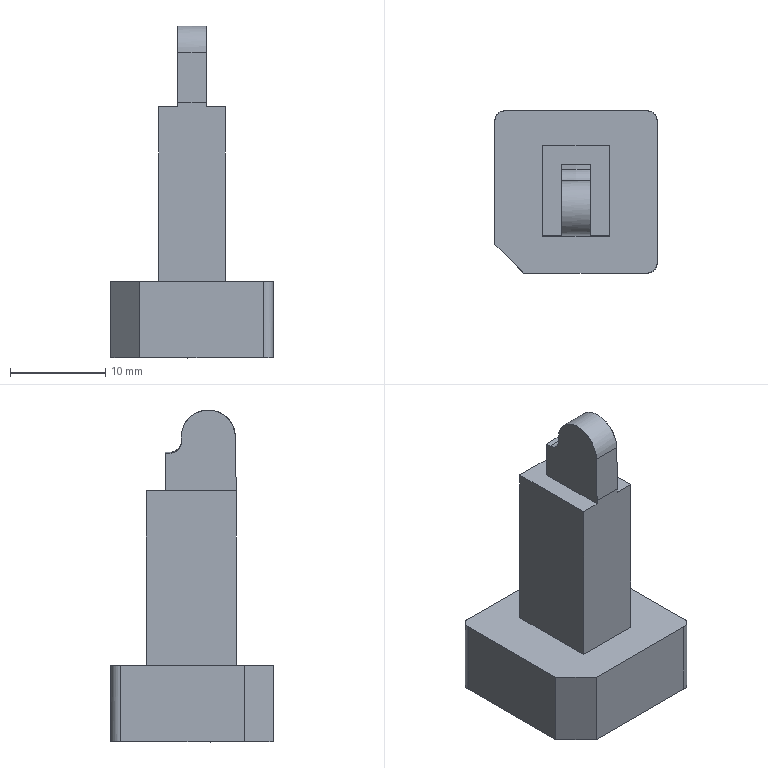NC program | PowerMill | posted with a generic post | part box 17 x 17 x 34.811 mm
Lines 6713 to 7479 of 35253:
N6810 M6
N6811 S18000 M03
N6812 G00 G90 X0.0 Y0.0
N6813 G43 Z10.798 H4
N6814
N6815 G05 P10000 R8
N6816 X1.6466 Y-5.3026
N6817 Z-2.4586
N6818 G01 Z-3.6586 F1200.0
N6819 X1.6444 Y-5.3048 Z-3.6763 F2000.0
N6820 X1.5692 Y-5.3292 Z-3.8957
N6821 X1.5752 Y-5.3231 Z-3.779
N6822 X1.587 Y-5.3114 Z-3.6547
N6823 X1.6045 Y-5.2939 Z-3.5284
N6824 X1.6264 Y-5.2719 Z-3.4092
N6825 X1.6518 Y-5.2466 Z-3.2995
N6826 X1.6598 Y-5.2386 Z-3.2691
N6827 X1.6694 Y-5.178 Z-3.0351
N6828 X1.6692 Y-5.1783 Z-3.0359
N6829 X1.635 Y-5.2125 Z-3.1368
N6830 X1.6045 Y-5.243 Z-3.245
N6831 X1.5779 Y-5.2696 Z-3.3607
N6832 X1.5553 Y-5.2921 Z-3.4838
N6833 X1.5372 Y-5.3102 Z-3.6141
N6834 X1.5238 Y-5.3236 Z-3.751
N6835 X1.5154 Y-5.332 Z-3.8931
N6836 X1.5123 Y-5.3352 Z-4.0382
N6837 X1.4611 Y-5.3355 Z-4.0525
N6838 X1.4638 Y-5.3327 Z-3.9138
N6839 X1.4717 Y-5.3248 Z-3.7684
N6840 X1.4849 Y-5.3117 Z-3.6241
N6841 X1.5029 Y-5.2936 Z-3.4852
N6842 X1.5253 Y-5.2712 Z-3.354
N6843 X1.5516 Y-5.2449 Z-3.2313
N6844 X1.5814 Y-5.2151 Z-3.1176
N6845 X1.6145 Y-5.1821 Z-3.0128
N6846 X1.6505 Y-5.1461 Z-2.9166
N6847 X1.6681 Y-5.1285 Z-2.8749
N6848 X1.6657 Y-5.0799 Z-2.7385
N6849 X1.6407 Y-5.1049 Z-2.7911
N6850 X1.6027 Y-5.1429 Z-2.8824
N6851 X1.5668 Y-5.1789 Z-2.9837
N6852 X1.5332 Y-5.2124 Z-3.0957
N6853 X1.5025 Y-5.2431 Z-3.2179
N6854 X1.4754 Y-5.2703 Z-3.3482
N6855 X1.4582 Y-5.2874 Z-3.447
N6856 X1.4406 Y-5.305 Z-3.5684
N6857 X1.4271 Y-5.3185 Z-3.6908
N6858 X1.4177 Y-5.328 Z-3.819
N6859 X1.4124 Y-5.3332 Z-3.9429
N6860 X1.4098 Y-5.3358 Z-4.0669
N6861 X1.3586 Y-5.3361 Z-4.0813
N6862 X1.3611 Y-5.3336 Z-3.9744
N6863 X1.3646 Y-5.3302 Z-3.8674
N6864 X1.3702 Y-5.3245 Z-3.7607
N6865 X1.3792 Y-5.3155 Z-3.6546
N6866 X1.392 Y-5.3028 Z-3.5494
N6867 X1.408 Y-5.2867 Z-3.445
N6868 X1.4262 Y-5.2685 Z-3.3433
N6869 X1.4553 Y-5.2394 Z-3.2034
N6870 X1.4875 Y-5.2073 Z-3.0738
N6871 X1.5223 Y-5.1724 Z-2.9551
N6872 X1.5596 Y-5.1351 Z-2.8467
N6873 X1.5994 Y-5.0953 Z-2.7478
N6874 X1.6416 Y-5.0531 Z-2.6579
N6875 X1.6679 Y-5.0269 Z-2.6085
N6876 X1.668 Y-4.9758 Z-2.495
N6877 X1.6354 Y-5.0084 Z-2.5489
N6878 X1.601 Y-5.0428 Z-2.6155
N6879 X1.5644 Y-5.0794 Z-2.6968
N6880 X1.5251 Y-5.1187 Z-2.7965
N6881 X1.4836 Y-5.1602 Z-2.9169
N6882 X1.4525 Y-5.1913 Z-3.0187
N6883 X1.4292 Y-5.2146 Z-3.1034
N6884 X1.4108 Y-5.233 Z-3.1767
N6885 X1.3834 Y-5.2604 Z-3.2999
N6886 X1.3599 Y-5.2839 Z-3.4246
N6887 X1.3407 Y-5.3031 Z-3.5529
N6888 X1.3255 Y-5.3183 Z-3.6908
N6889 X1.3154 Y-5.3284 Z-3.8285
N6890 X1.3099 Y-5.3339 Z-3.9605
N6891 X1.3076 Y-5.3362 Z-4.0898
N6892 X1.2567
N6893 X1.2589 Y-5.334 Z-3.9688
N6894 X1.2633 Y-5.3296 Z-3.8479
N6895 X1.271 Y-5.3219 Z-3.7274
N6896 X1.2838 Y-5.3091 Z-3.5979
N6897 X1.3003 Y-5.2926 Z-3.4794
N6898 X1.3208 Y-5.2721 Z-3.3621
N6899 X1.3446 Y-5.2483 Z-3.246
N6900 X1.363 Y-5.2298 Z-3.1654
N6901 X1.3865 Y-5.2064 Z-3.0737
N6902 X1.4171 Y-5.1758 Z-2.9669
N6903 X1.4568 Y-5.1361 Z-2.8437
N6904 X1.5011 Y-5.0918 Z-2.7224
N6905 X1.5437 Y-5.0492 Z-2.6196
N6906 X1.5843 Y-5.0086 Z-2.5333
N6907 X1.6232 Y-4.9697 Z-2.461
N6908 X1.6624 Y-4.9305 Z-2.398
N6909 X1.6671 Y-4.9257 Z-2.3911
N6910 X1.6656 Y-4.8764 Z-2.2976
N6911 X1.665 Y-4.877 Z-2.2984
N6912 X1.6183 Y-4.9237 Z-2.3674
N6913 X1.5741 Y-4.9679 Z-2.4436
N6914 X1.5311 Y-5.0109 Z-2.5294
N6915 X1.4887 Y-5.0533 Z-2.626
N6916 X1.4466 Y-5.0954 Z-2.734
N6917 X1.4066 Y-5.1354 Z-2.8455
N6918 X1.3673 Y-5.1746 Z-2.9639
N6919 X1.3296 Y-5.2124 Z-3.0941
N6920 X1.2969 Y-5.2451 Z-3.2267
N6921 X1.2697 Y-5.2723 Z-3.3598
N6922 X1.2498 Y-5.2921 Z-3.4775
N6923 X1.2335 Y-5.3085 Z-3.5963
N6924 X1.2212 Y-5.3208 Z-3.716
N6925 X1.2125 Y-5.3295 Z-3.8476
N6926 X1.2081 Y-5.3339 Z-3.9687
N6927 X1.2057 Y-5.3362 Z-4.0898
N6928 X1.1548
N6929 X1.1573 Y-5.3338 Z-3.9582
N6930 X1.1629 Y-5.3282 Z-3.8268
N6931 X1.173 Y-5.318 Z-3.6892
N6932 X1.1885 Y-5.3026 Z-3.5501
N6933 X1.2078 Y-5.2833 Z-3.4215
N6934 X1.2315 Y-5.2595 Z-3.2944
N6935 X1.2592 Y-5.2318 Z-3.1689
N6936 X1.2768 Y-5.2143 Z-3.0988
N6937 X1.2975 Y-5.1936 Z-3.0249
N6938 X1.324 Y-5.1671 Z-2.9386
N6939 X1.3581 Y-5.133 Z-2.837
N6940 X1.4025 Y-5.0886 Z-2.7159
N6941 X1.4551 Y-5.0359 Z-2.5865
N6942 X1.5027 Y-4.9884 Z-2.4812
N6943 X1.5458 Y-4.9453 Z-2.3951
N6944 X1.5855 Y-4.9056 Z-2.3242
N6945 X1.6223 Y-4.8688 Z-2.2658
N6946 X1.6598 Y-4.8312 Z-2.2145
N6947 X1.6649 Y-4.8262 Z-2.2082
N6948 X1.6632 Y-4.7769 Z-2.1258
N6949 X1.6337 Y-4.8065 Z-2.1622
N6950 X1.5966 Y-4.8435 Z-2.2145
N6951 X1.5568 Y-4.8834 Z-2.2784
N6952 X1.5137 Y-4.9265 Z-2.3556
N6953 X1.4665 Y-4.9736 Z-2.4491
N6954 X1.4143 Y-5.0259 Z-2.5636
N6955 X1.3581 Y-5.0821 Z-2.7001
N6956 X1.3143 Y-5.1258 Z-2.817
N6957 X1.2804 Y-5.1598 Z-2.916
N6958 X1.2537 Y-5.1865 Z-3.001
N6959 X1.2327 Y-5.2075 Z-3.0742
N6960 X1.2147 Y-5.2255 Z-3.1445
N6961 X1.1853 Y-5.2548 Z-3.2735
N6962 X1.1601 Y-5.2801 Z-3.4041
N6963 X1.1392 Y-5.301 Z-3.5386
N6964 X1.1229 Y-5.3173 Z-3.6796
N6965 X1.1121 Y-5.3281 Z-3.8188
N6966 X1.1061 Y-5.334 Z-3.9543
N6967 X1.1039 Y-5.3362 Z-4.0898
N6968 X1.053
N6969 X1.0552 Y-5.334 Z-3.961
N6970 X1.0605 Y-5.3288 Z-3.8322
N6971 X1.0699 Y-5.3194 Z-3.6999
N6972 X1.0844 Y-5.3048 Z-3.5639
N6973 X1.1041 Y-5.2851 Z-3.4306
N6974 X1.1278 Y-5.2614 Z-3.3046
N6975 X1.1555 Y-5.2338 Z-3.182
N6976 X1.1869 Y-5.2024 Z-3.0612
N6977 X1.2216 Y-5.1676 Z-2.9423
N6978 X1.2672 Y-5.1221 Z-2.8057
N6979 X1.3188 Y-5.0705 Z-2.6693
N6980 X1.3766 Y-5.0127 Z-2.5333
N6981 X1.4407 Y-4.9486 Z-2.3978
N6982 X1.4658 Y-4.9235 Z-2.3488
N6983 X1.4951 Y-4.8942 Z-2.2947
N6984 X1.5364 Y-4.8528 Z-2.2233
N6985 X1.5812 Y-4.8081 Z-2.1524
N6986 X1.6165 Y-4.7728 Z-2.1021
N6987 X1.6484 Y-4.7409 Z-2.0623
N6988 X1.6615 Y-4.7278 Z-2.0479
N6989 X1.6662 Y-4.6721 Z-1.9658
N6990 X1.6558 Y-4.6826 Z-1.9778
N6991 X1.6131 Y-4.7252 Z-2.0286
N6992 X1.5722 Y-4.7661 Z-2.0821
N6993 X1.5337 Y-4.8046 Z-2.1391
N6994 X1.4978 Y-4.8406 Z-2.1996
N6995 X1.4634 Y-4.875 Z-2.262
N6996 X1.4294 Y-4.9089 Z-2.3249
N6997 X1.3887 Y-4.9497 Z-2.4028
N6998 X1.3262 Y-5.0121 Z-2.5326
N6999 X1.2694 Y-5.069 Z-2.6647
N7000 X1.2182 Y-5.1201 Z-2.7985
N7001 X1.1728 Y-5.1656 Z-2.9339
N7002 X1.1377 Y-5.2007 Z-3.0535
N7003 X1.1061 Y-5.2323 Z-3.175
N7004 X1.0782 Y-5.2602 Z-3.2983
N7005 X1.0543 Y-5.284 Z-3.4244
N7006 X1.0344 Y-5.3039 Z-3.5579
N7007 X1.0195 Y-5.3188 Z-3.6955
N7008 X1.0098 Y-5.3285 Z-3.8297
N7009 X1.0044 Y-5.334 Z-3.9602
N7010 X1.0021 Y-5.3362 Z-4.0898
N7011 X0.9512
N7012 X0.9537 Y-5.3337 Z-3.9469
N7013 X0.9604 Y-5.327 Z-3.8049
N7014 X0.9718 Y-5.3156 Z-3.6636
N7015 X0.9885 Y-5.2989 Z-3.5231
N7016 X1.0107 Y-5.2768 Z-3.3835
N7017 X1.0381 Y-5.2494 Z-3.2468
N7018 X1.0704 Y-5.217 Z-3.113
N7019 X1.1074 Y-5.1801 Z-2.9819
N7020 X1.1487 Y-5.1387 Z-2.8524
N7021 X1.1968 Y-5.0906 Z-2.7196
N7022 X1.2512 Y-5.0362 Z-2.5867
N7023 X1.3117 Y-4.9757 Z-2.4541
N7024 X1.3769 Y-4.9105 Z-2.3237
N7025 X1.4393 Y-4.8481 Z-2.2105
N7026 X1.4887 Y-4.7987 Z-2.1293
N7027 X1.548 Y-4.7394 Z-2.0394
N7028 X1.5981 Y-4.6893 Z-1.9714
N7029 X1.6448 Y-4.6426 Z-1.9169
N7030 X1.6687 Y-4.6187 Z-1.8926
N7031 X1.6718 Y-4.5648 Z-1.8222
N7032 X1.6649 Y-4.5716 Z-1.8284
N7033 X1.6207 Y-4.6158 Z-1.8729
N7034 X1.5719 Y-4.6646 Z-1.9311
N7035 X1.5195 Y-4.717 Z-2.003
N7036 X1.4778 Y-4.7587 Z-2.0661
N7037 X1.4417 Y-4.7948 Z-2.1243
N7038 X1.4064 Y-4.8301 Z-2.1831
N7039 X1.3329 Y-4.9036 Z-2.3132
N7040 X1.2656 Y-4.9709 Z-2.4447
N7041 X1.2045 Y-5.032 Z-2.5773
N7042 X1.1494 Y-5.0871 Z-2.711
N7043 X1.1002 Y-5.1363 Z-2.8457
N7044 X1.0582 Y-5.1784 Z-2.9763
N7045 X1.0208 Y-5.2157 Z-3.1081
N7046 X0.9881 Y-5.2484 Z-3.2425
N7047 X0.9605 Y-5.276 Z-3.3796
N7048 X0.9381 Y-5.2984 Z-3.5194
N7049 X0.9213 Y-5.3153 Z-3.6604
N7050 X0.9096 Y-5.3269 Z-3.8025
N7051 X0.9028 Y-5.3337 Z-3.9456
N7052 X0.9003 Y-5.3362 Z-4.0898
N7053 X0.8494
N7054 X0.8516 Y-5.334 Z-3.9643
N7055 X0.8565 Y-5.3291 Z-3.839
N7056 X0.8656 Y-5.32 Z-3.7075
N7057 X0.8796 Y-5.306 Z-3.5748
N7058 X0.8973 Y-5.2883 Z-3.4521
N7059 X0.9193 Y-5.2663 Z-3.3307
N7060 X0.9449 Y-5.2407 Z-3.2107
N7061 X0.9798 Y-5.2058 Z-3.0712
N7062 X1.0204 Y-5.1652 Z-2.9328
N7063 X1.0667 Y-5.1189 Z-2.7955
N7064 X1.1188 Y-5.0668 Z-2.6597
N7065 X1.1766 Y-5.009 Z-2.5254
N7066 X1.2402 Y-4.9454 Z-2.393
N7067 X1.3095 Y-4.8761 Z-2.2628
N7068 X1.3845 Y-4.8011 Z-2.1351
N7069 X1.4501 Y-4.7355 Z-2.0313
N7070 X1.5081 Y-4.6775 Z-1.945
N7071 X1.5607 Y-4.6249 Z-1.8745
N7072 X1.6104 Y-4.5752 Z-1.8168
N7073 X1.6589 Y-4.5267 Z-1.7696
N7074 X1.675 Y-4.5106 Z-1.756
N7075 X1.6805 Y-4.4542 Z-1.6882
N7076 X1.6609 Y-4.4738 Z-1.7045
N7077 X1.6112 Y-4.5235 Z-1.7517
N7078 X1.5585 Y-4.5762 Z-1.8104
N7079 X1.5014 Y-4.6333 Z-1.8832
N7080 X1.4367 Y-4.698 Z-1.9749
N7081 X1.3569 Y-4.7778 Z-2.0976
N7082 X1.2882 Y-4.8465 Z-2.2108
N7083 X1.2167 Y-4.918 Z-2.3398
N7084 X1.1509 Y-4.9838 Z-2.4714
N7085 X1.0907 Y-5.044 Z-2.6053
N7086 X1.036 Y-5.0987 Z-2.7413
N7087 X0.9871 Y-5.1476 Z-2.8791
N7088 X0.9437 Y-5.191 Z-3.0185
N7089 X0.906 Y-5.2287 Z-3.1591
N7090 X0.8741 Y-5.2606 Z-3.3006
N7091 X0.8478 Y-5.2869 Z-3.4426
N7092 X0.8297 Y-5.305 Z-3.5663
N7093 X0.8161 Y-5.3186 Z-3.6912
N7094 X0.8066 Y-5.3281 Z-3.8235
N7095 X0.801 Y-5.3337 Z-3.9633
N7096 X0.7985 Y-5.3362 Z-4.0898
N7097 X0.7476
N7098 X0.7499 Y-5.3339 Z-3.9655
N7099 X0.7547 Y-5.3291 Z-3.8412
N7100 X0.7637 Y-5.3201 Z-3.7091
N7101 X0.7775 Y-5.3062 Z-3.5758
N7102 X0.795 Y-5.2888 Z-3.4541
N7103 X0.8166 Y-5.2672 Z-3.3338
N7104 X0.842 Y-5.2418 Z-3.2149
N7105 X0.8761 Y-5.2077 Z-3.078
N7106 X0.9154 Y-5.1684 Z-2.9426
N7107 X0.9603 Y-5.1234 Z-2.8081
N7108 X1.0113 Y-5.0725 Z-2.6741
N7109 X1.0686 Y-5.0152 Z-2.54
N7110 X1.1324 Y-4.9513 Z-2.4056
N7111 X1.1903 Y-4.8935 Z-2.2939
N7112 X1.2177 Y-4.866 Z-2.2442
N7113 X1.2471 Y-4.8367 Z-2.1935
N7114 X1.2836 Y-4.8001 Z-2.1328
N7115 X1.3296 Y-4.7541 Z-2.0597
N7116 X1.39 Y-4.6938 Z-1.9686
N7117 X1.4623 Y-4.6215 Z-1.8671
N7118 X1.5204 Y-4.5633 Z-1.7921
N7119 X1.5697 Y-4.5141 Z-1.7341
N7120 X1.6127 Y-4.4711 Z-1.6886
N7121 X1.6505 Y-4.4332 Z-1.6535
N7122 X1.6846 Y-4.3991 Z-1.6271
N7123 X1.6869 Y-4.346 Z-1.5698
N7124 X1.6537 Y-4.3792 Z-1.594
N7125 X1.6038 Y-4.4291 Z-1.6373
N7126 X1.5521 Y-4.4808 Z-1.6908
N7127 X1.4949 Y-4.5379 Z-1.759
N7128 X1.4367 Y-4.5962 Z-1.8342
N7129 X1.3515 Y-4.6813 Z-1.951
N7130 X1.2688 Y-4.7641 Z-2.0746
N7131 X1.1928 Y-4.8401 Z-2.1992
N7132 X1.1379 Y-4.895 Z-2.2974
N7133 X1.0856 Y-4.9473 Z-2.3985
N7134 X1.0305 Y-5.0024 Z-2.5128
N7135 X0.9832 Y-5.0497 Z-2.6186
N7136 X0.9393 Y-5.0936 Z-2.7274
N7137 X0.8895 Y-5.1434 Z-2.8662
N7138 X0.8454 Y-5.1874 Z-3.0062
N7139 X0.8072 Y-5.2257 Z-3.1471
N7140 X0.7747 Y-5.2582 Z-3.2886
N7141 X0.7479 Y-5.2849 Z-3.4304
N7142 X0.7292 Y-5.3037 Z-3.5556
N7143 X0.7151 Y-5.3177 Z-3.682
N7144 X0.7056 Y-5.3272 Z-3.8093
N7145 X0.6993 Y-5.3336 Z-3.9585
N7146 X0.6966 Y-5.3362 Z-4.0898
N7147 X0.6457
N7148 X0.6482 Y-5.3338 Z-3.9424
N7149 X0.6553 Y-5.3267 Z-3.7967
N7150 X0.6674 Y-5.3146 Z-3.6526
N7151 X0.6848 Y-5.2971 Z-3.5101
N7152 X0.7076 Y-5.2743 Z-3.3702
N7153 X0.7357 Y-5.2463 Z-3.233
N7154 X0.7688 Y-5.2132 Z-3.0984
N7155 X0.8066 Y-5.1753 Z-2.966
N7156 X0.8493 Y-5.1327 Z-2.8346
N7157 X0.8978 Y-5.0842 Z-2.7034
N7158 X0.9533 Y-5.0287 Z-2.5701
N7159 X1.0162 Y-4.9658 Z-2.4344
N7160 X1.0856 Y-4.8963 Z-2.299
N7161 X1.1594 Y-4.8225 Z-2.1687
N7162 X1.2374 Y-4.7446 Z-2.0438
N7163 X1.3192 Y-4.6628 Z-1.9246
N7164 X1.4056 Y-4.5764 Z-1.8075
N7165 X1.4818 Y-4.5002 Z-1.7128
N7166 X1.5472 Y-4.4347 Z-1.6384
N7167 X1.6026 Y-4.3793 Z-1.5827
N7168 X1.6537 Y-4.3282 Z-1.5393
N7169 X1.685 Y-4.2969 Z-1.5168
N7170 X1.6834 Y-4.2477 Z-1.4676
N7171 X1.6744 Y-4.2566 Z-1.4735
N7172 X1.6218 Y-4.3093 Z-1.5129
N7173 X1.5658 Y-4.3652 Z-1.5633
N7174 X1.5033 Y-4.4277 Z-1.6281
N7175 X1.4576 Y-4.4734 Z-1.6806
N7176 X1.4022 Y-4.5289 Z-1.7484
N7177 X1.3474 Y-4.5836 Z-1.8174
N7178 X1.2714 Y-4.6596 Z-1.9203
N7179 X1.1912 Y-4.7398 Z-2.0378
N7180 X1.1211 Y-4.81 Z-2.1488
N7181 X1.0564 Y-4.8747 Z-2.2596
N7182 X0.9875 Y-4.9436 Z-2.3894
N7183 X0.9234 Y-5.0076 Z-2.523
N7184 X0.8649 Y-5.0662 Z-2.6591
N7185 X0.8122 Y-5.1189 Z-2.7964
N7186 X0.7656 Y-5.1655 Z-2.9341
N7187 X0.7252 Y-5.2059 Z-3.0713
N7188 X0.691 Y-5.2401 Z-3.2074
N7189 X0.6652 Y-5.2658 Z-3.3279
N7190 X0.6431 Y-5.2879 Z-3.4498
N7191 X0.6253 Y-5.3058 Z-3.5731
N7192 X0.6112 Y-5.3199 Z-3.7061
N7193 X0.602 Y-5.329 Z-3.8379
N7194 X0.5971 Y-5.334 Z-3.9638
N7195 X0.5948 Y-5.3362 Z-4.0898
N7196 X0.5439
N7197 X0.5463 Y-5.3339 Z-3.9681
N7198 X0.5508 Y-5.3293 Z-3.8465
N7199 X0.5587 Y-5.3214 Z-3.7243
N7200 X0.5707 Y-5.3094 Z-3.6039
N7201 X0.5869 Y-5.2933 Z-3.4845
N7202 X0.6067 Y-5.2734 Z-3.3662
N7203 X0.6301 Y-5.25 Z-3.2492
N7204 X0.6584 Y-5.2217 Z-3.1316
N7205 X0.6947 Y-5.1854 Z-3.0011
N7206 X0.7406 Y-5.1395 Z-2.8565
N7207 X0.7859 Y-5.0943 Z-2.7295
N7208 X0.8287 Y-5.0515 Z-2.6209
N7209 X0.863 Y-5.0171 Z-2.5415
N7210 X0.8999 Y-4.9802 Z-2.4646
N7211 X0.9383 Y-4.9418 Z-2.3891
N7212 X0.9902 Y-4.89 Z-2.2917
N7213 X1.0307 Y-4.8494 Z-2.2184
N7214 X1.0723 Y-4.8079 Z-2.1463
N7215 X1.1155 Y-4.7646 Z-2.0762
N7216 X1.2036 Y-4.6765 Z-1.9444
N7217 X1.2926 Y-4.5876 Z-1.8224
N7218 X1.3825 Y-4.4977 Z-1.7097
N7219 X1.4223 Y-4.4578 Z-1.663
N7220 X1.4625 Y-4.4176 Z-1.6168
N7221 X1.5032 Y-4.3769 Z-1.5713
N7222 X1.5466 Y-4.3335 Z-1.5261
N7223 X1.5977 Y-4.2824 Z-1.4794
N7224 X1.643 Y-4.2371 Z-1.4446
N7225 X1.6812 Y-4.199 Z-1.4193
N7226 X1.6791 Y-4.1501 Z-1.3727
N7227 X1.6749 Y-4.1543 Z-1.3751
N7228 X1.6427 Y-4.1865 Z-1.3966
N7229 X1.6097 Y-4.2195 Z-1.4223
N7230 X1.5658 Y-4.2634 Z-1.46
N7231 X1.5121 Y-4.3171 Z-1.5098
N7232 X1.4762 Y-4.353 Z-1.5452
N7233 X1.4474 Y-4.3818 Z-1.5751
N7234 X1.4193 Y-4.41 Z-1.6062
N7235 X1.3454 Y-4.4838 Z-1.6929
N7236 X1.2734 Y-4.5559 Z-1.7827
N7237 X1.188 Y-4.6412 Z-1.8955
N7238 X1.12 Y-4.7092 Z-1.9913
N7239 X1.0545 Y-4.7747 Z-2.0905
N7240 X0.9817 Y-4.8475 Z-2.2118
N7241 X0.9087 Y-4.9205 Z-2.3455
N7242 X0.8423 Y-4.987 Z-2.4795
N7243 X0.7817 Y-5.0475 Z-2.6146
N7244 X0.7273 Y-5.1019 Z-2.7502
N7245 X0.6789 Y-5.1503 Z-2.8865
N7246 X0.6364 Y-5.1929 Z-3.0236
N7247 X0.5995 Y-5.2297 Z-3.1618
N7248 X0.5683 Y-5.2609 Z-3.3011
N7249 X0.5426 Y-5.2866 Z-3.4417
N7250 X0.5223 Y-5.3069 Z-3.5837
N7251 X0.509 Y-5.3202 Z-3.7094
N7252 X0.5002 Y-5.3291 Z-3.8358
N7253 X0.4953 Y-5.3339 Z-3.9627
N7254 X0.493 Y-5.3362 Z-4.0898
N7255 X0.4421
N7256 X0.4444 Y-5.3339 Z-3.9585
N7257 X0.4501 Y-5.3282 Z-3.8233
N7258 X0.4606 Y-5.3177 Z-3.6835
N7259 X0.4762 Y-5.3021 Z-3.5453
N7260 X0.496 Y-5.2824 Z-3.4157
N7261 X0.5199 Y-5.2584 Z-3.29
N7262 X0.5479 Y-5.2304 Z-3.1661
N7263 X0.5799 Y-5.1984 Z-3.044
N7264 X0.6212 Y-5.1571 Z-2.9074
N7265 X0.6687 Y-5.1096 Z-2.7707
N7266 X0.7224 Y-5.0559 Z-2.6339
N7267 X0.7825 Y-4.9958 Z-2.4971
N7268 X0.8472 Y-4.9311 Z-2.3647
N7269 X0.9158 Y-4.8625 Z-2.2382
N7270 X0.9856 Y-4.7927 Z-2.1213
N7271 X1.058 Y-4.7203 Z-2.0075
N7272 X1.1335 Y-4.6448 Z-1.8979
N7273 X1.2124 Y-4.5659 Z-1.7932
N7274 X1.2941 Y-4.4842 Z-1.6929
N7275 X1.3608 Y-4.4175 Z-1.615
N7276 X1.4433 Y-4.335 Z-1.5244
N7277 X1.5141 Y-4.2642 Z-1.4542
N7278 X1.5786 Y-4.1997 Z-1.3962
N7279 X1.6282 Y-4.1501 Z-1.3572
N7280 X1.6721 Y-4.1062 Z-1.3297
N7281 X1.678 Y-4.1003 Z-1.3266
N7282 X1.6757 Y-4.0517 Z-1.2848
N7283 X1.6719 Y-4.0555 Z-1.287
N7284 X1.6158 Y-4.1116 Z-1.3234
N7285 X1.5563 Y-4.1711 Z-1.3698
N7286 X1.4924 Y-4.235 Z-1.4272
N7287 X1.4223 Y-4.3051 Z-1.4968
N7288 X1.3439 Y-4.3835 Z-1.5798
N7289 X1.2503 Y-4.4771 Z-1.6854
N7290 X1.1552 Y-4.5722 Z-1.8024
N7291 X1.0647 Y-4.6627 Z-1.9243
N7292 X0.9789 Y-4.7485 Z-2.0508
N7293 X0.8992 Y-4.8282 Z-2.1794
N7294 X0.8253 Y-4.9021 Z-2.3105
N7295 X0.7571 Y-4.9703 Z-2.4438
N7296 X0.6947 Y-5.0327 Z-2.5792
N7297 X0.6381 Y-5.0893 Z-2.7164
N7298 X0.5914 Y-5.136 Z-2.8433
N7299 X0.5491 Y-5.1783 Z-2.9751
N7300 X0.5108 Y-5.2166 Z-3.1134
N7301 X0.4828 Y-5.2446 Z-3.23
N7302 X0.4579 Y-5.2695 Z-3.348
N7303 X0.4366 Y-5.2908 Z-3.4673
N7304 X0.4194 Y-5.3079 Z-3.588
N7305 X0.4059 Y-5.3215 Z-3.7207
N7306 X0.3979 Y-5.3295 Z-3.8434
N7307 X0.3933 Y-5.3341 Z-3.9666
N7308 X0.3912 Y-5.3362 Z-4.0898
N7309 X0.3403
N7310 X0.3426 Y-5.3339 Z-3.9611
N7311 X0.3477 Y-5.3288 Z-3.8321
N7312 X0.3567 Y-5.3198 Z-3.7042
N7313 X0.3703 Y-5.3062 Z-3.5771
N7314 X0.3883 Y-5.2882 Z-3.4511
N7315 X0.4138 Y-5.2627 Z-3.3106
N7316 X0.4449 Y-5.2316 Z-3.1705
N7317 X0.4818 Y-5.1947 Z-3.031
N7318 X0.5244 Y-5.1521 Z-2.8923
N7319 X0.5729 Y-5.1036 Z-2.7546
N7320 X0.6272 Y-5.0493 Z-2.6182
N7321 X0.6872 Y-4.9892 Z-2.4833
N7322 X0.7531 Y-4.9234 Z-2.3502
N7323 X0.8247 Y-4.8518 Z-2.2195
N7324 X0.9019 Y-4.7745 Z-2.0914
N7325 X0.9841 Y-4.6924 Z-1.9669
N7326 X1.0733 Y-4.6031 Z-1.843
N7327 X1.1674 Y-4.5091 Z-1.7234
N7328 X1.2665 Y-4.4099 Z-1.6081
N7329 X1.3488 Y-4.3277 Z-1.5197
N7330 X1.3917 Y-4.2847 Z-1.4755
N7331 X1.4353 Y-4.2412 Z-1.4323
N7332 X1.49 Y-4.1865 Z-1.3807
N7333 X1.5591 Y-4.1174 Z-1.3212
N7334 X1.6143 Y-4.0622 Z-1.2796
N7335 X1.6625 Y-4.014 Z-1.2492
N7336 X1.6741 Y-4.0024 Z-1.2428
N7337 X1.674 Y-3.9516 Z-1.2004
N7338 X1.63 Y-3.9956 Z-1.2242
N7339 X1.5782 Y-4.0474 Z-1.2599
N7340 X1.5139 Y-4.1117 Z-1.3115
N7341 X1.4388 Y-4.1868 Z-1.3783
N7342 X1.3486 Y-4.277 Z-1.4669
N7343 X1.2445 Y-4.3811 Z-1.5755
N7344 X1.1441 Y-4.4814 Z-1.6898
N7345 X1.0477 Y-4.5779 Z-1.8097
N7346 X0.9554 Y-4.6702 Z-1.9351
N7347 X0.8705 Y-4.7551 Z-2.061
N7348 X0.7916 Y-4.834 Z-2.1889
N7349 X0.7187 Y-4.9069 Z-2.3188
N7350 X0.6519 Y-4.9737 Z-2.4505
N7351 X0.5909 Y-5.0346 Z-2.5837
N7352 X0.5359 Y-5.0897 Z-2.7183
N7353 X0.4866 Y-5.1389 Z-2.8545
N7354 X0.4504 Y-5.1752 Z-2.9653
N7355 X0.4172 Y-5.2083 Z-3.0781
N7356 X0.3883 Y-5.2372 Z-3.1931
N7357 X0.3636 Y-5.2619 Z-3.31
N7358 X0.3437 Y-5.2819 Z-3.4192
N7359 X0.3261 Y-5.2995 Z-3.5291
N7360 X0.3118 Y-5.3138 Z-3.6399
N7361 X0.3015 Y-5.324 Z-3.7517
N7362 X0.2951 Y-5.3304 Z-3.8642
N7363 X0.2915 Y-5.3341 Z-3.977
N7364 X0.2893 Y-5.3362 Z-4.0898
N7365 X0.2384
N7366 X0.2407 Y-5.3339 Z-3.9609
N7367 X0.246 Y-5.3286 Z-3.8322
N7368 X0.2557 Y-5.319 Z-3.6974
N7369 X0.2707 Y-5.304 Z-3.5595
N7370 X0.2896 Y-5.285 Z-3.4318
N7371 X0.3128 Y-5.2619 Z-3.3073
N7372 X0.3399 Y-5.2347 Z-3.1844
N7373 X0.3708 Y-5.2039 Z-3.0632
N7374 X0.4092 Y-5.1655 Z-2.9336
N7375 X0.4549 Y-5.1197 Z-2.799
N7376 X0.5079 Y-5.0668 Z-2.6611
N7377 X0.5673 Y-5.0074 Z-2.5228
N7378 X0.6305 Y-4.9441 Z-2.3904
N7379 X0.6949 Y-4.8798 Z-2.2684
N7380 X0.7601 Y-4.8146 Z-2.1561
N7381 X0.8428 Y-4.7318 Z-2.0254
N7382 X0.9307 Y-4.644 Z-1.8987
N7383 X1.0234 Y-4.5512 Z-1.7761
N7384 X1.122 Y-4.4526 Z-1.6566
N7385 X1.2255 Y-4.3491 Z-1.5417
N7386 X1.3338 Y-4.2409 Z-1.4316
N7387 X1.4095 Y-4.1652 Z-1.3601
N7388 X1.4639 Y-4.1108 Z-1.3112
N7389 X1.5373 Y-4.0373 Z-1.2498
N7390 X1.5975 Y-3.9771 Z-1.2059
N7391 X1.6487 Y-3.9259 Z-1.1748
N7392 X1.6753 Y-3.8994 Z-1.1616
N7393 X1.677 Y-3.8468 Z-1.1223
N7394 X1.6506 Y-3.8732 Z-1.1349
N7395 X1.5928 Y-3.931 Z-1.1683
N7396 X1.5291 Y-3.9947 Z-1.2132
N7397 X1.4535 Y-4.0703 Z-1.2743
N7398 X1.3608 Y-4.163 Z-1.3571
N7399 X1.2509 Y-4.2728 Z-1.4637
N7400 X1.1646 Y-4.3592 Z-1.553
N7401 X1.0739 Y-4.4499 Z-1.6543
N7402 X0.9754 Y-4.5483 Z-1.7733
N7403 X0.8845 Y-4.6393 Z-1.8925
N7404 X0.8057 Y-4.718 Z-2.0043
N7405 X0.7305 Y-4.7932 Z-2.121
N7406 X0.654 Y-4.8697 Z-2.2511
N7407 X0.5835 Y-4.9403 Z-2.3833
N7408 X0.5186 Y-5.0052 Z-2.5178
N7409 X0.4599 Y-5.0639 Z-2.6531
N7410 X0.4073 Y-5.1164 Z-2.789
N7411 X0.3609 Y-5.1629 Z-2.9252
N7412 X0.3204 Y-5.2034 Z-3.0618
N7413 X0.2895 Y-5.2343 Z-3.1825
N7414 X0.2623 Y-5.2614 Z-3.305
N7415 X0.2391 Y-5.2846 Z-3.429
N7416 X0.2201 Y-5.3036 Z-3.5566
N7417 X0.2051 Y-5.3187 Z-3.6941
N7418 X0.1952 Y-5.3285 Z-3.8307
N7419 X0.1898 Y-5.3339 Z-3.9613
N7420 X0.1875 Y-5.3362 Z-4.0898
N7421 X0.1366
N7422 X0.1389 Y-5.3339 Z-3.9565
N7423 X0.1449 Y-5.328 Z-3.8195
N7424 X0.1556 Y-5.3173 Z-3.6787
N7425 X0.1713 Y-5.3015 Z-3.5407
N7426 X0.1913 Y-5.2815 Z-3.4109
N7427 X0.2154 Y-5.2574 Z-3.2854
N7428 X0.2437 Y-5.2291 Z-3.1616
N7429 X0.2758 Y-5.197 Z-3.0398
N7430 X0.3179 Y-5.1549 Z-2.9013
N7431 X0.3658 Y-5.1071 Z-2.764
N7432 X0.4194 Y-5.0534 Z-2.6279
N7433 X0.4789 Y-4.994 Z-2.4932
N7434 X0.5442 Y-4.9286 Z-2.3603
N7435 X0.6154 Y-4.8574 Z-2.2293
N7436 X0.6925 Y-4.7804 Z-2.1005
N7437 X0.7753 Y-4.6976 Z-1.9744
N7438 X0.8639 Y-4.6089 Z-1.851
N7439 X0.9589 Y-4.5139 Z-1.7299
N7440 X1.0603 Y-4.4125 Z-1.6111
N7441 X1.1597 Y-4.3131 Z-1.504
N7442 X1.2665 Y-4.2063 Z-1.3985
N7443 X1.3872 Y-4.0856 Z-1.2884
N7444 X1.4436 Y-4.0292 Z-1.2396
N7445 X1.5173 Y-3.9555 Z-1.1803
N7446 X1.5845 Y-3.8883 Z-1.1338
N7447 X1.6477 Y-3.8251 Z-1.0979
N7448 X1.6784 Y-3.7945 Z-1.0833
N7449 X1.6788 Y-3.7431 Z-1.0493
N7450 X1.6706 Y-3.7514 Z-1.0525
N7451 X1.619 Y-3.8029 Z-1.0767
N7452 X1.5607 Y-3.8613 Z-1.1118
N7453 X1.4895 Y-3.9324 Z-1.162
N7454 X1.4087 Y-4.0132 Z-1.2257
N7455 X1.3113 Y-4.1106 Z-1.3105
N7456 X1.1961 Y-4.2258 Z-1.4171
N7457 X1.0865 Y-4.3355 Z-1.5273
N7458 X0.9825 Y-4.4394 Z-1.6414
N7459 X0.8842 Y-4.5377 Z-1.759
N7460 X0.7911 Y-4.6308 Z-1.8805
N7461 X0.703 Y-4.7189 Z-2.0061
N7462 X0.6212 Y-4.8008 Z-2.1337
N7463 X0.5455 Y-4.8765 Z-2.2632
N7464 X0.4758 Y-4.9461 Z-2.3945
N7465 X0.4121 Y-5.0098 Z-2.5274
N7466 X0.3543 Y-5.0676 Z-2.6618
N7467 X0.3024 Y-5.1196 Z-2.7978
N7468 X0.2561 Y-5.1659 Z-2.9351
N7469 X0.2154 Y-5.2065 Z-3.0738
N7470 X0.1801 Y-5.2418 Z-3.2149
N7471 X0.1548 Y-5.2672 Z-3.3336
N7472 X0.1331 Y-5.2888 Z-3.4538
N7473 X0.1158 Y-5.3062 Z-3.5753
N7474 X0.1019 Y-5.32 Z-3.7083
N7475 X0.0929 Y-5.329 Z-3.8415
N7476 X0.088 Y-5.3339 Z-3.9656
N7477 X0.0857 Y-5.3362 Z-4.0898
N7478 X0.0348
N7479 X0.0371 Y-5.3339 Z-3.9658
N7480 X0.042 Y-5.329 Z-3.8419
N7481 X0.051 Y-5.3201 Z-3.7087
N7482 X0.0648 Y-5.3062 Z-3.5758
N7483 X0.0821 Y-5.2889 Z-3.4545
N7484 X0.1037 Y-5.2674 Z-3.3345
N7485 X0.129 Y-5.242 Z-3.216
N7486 X0.1643 Y-5.2067 Z-3.0748
N7487 X0.205 Y-5.166 Z-2.9358
N7488 X0.2513 Y-5.1197 Z-2.7983
N7489 X0.3033 Y-5.0677 Z-2.6622
N7490 X0.3611 Y-5.0099 Z-2.5277
N7491 X0.4247 Y-4.9463 Z-2.3948
N7492 X0.4943 Y-4.8768 Z-2.2636
N7493 X0.5698 Y-4.8012 Z-2.1344
N7494 X0.6514 Y-4.7196 Z-2.0072
N7495 X0.7391 Y-4.6319 Z-1.8822
N7496 X0.8248 Y-4.5462 Z-1.7698
N7497 X0.9196 Y-4.4514 Z-1.6548
N7498 X1.0188 Y-4.3522 Z-1.5443
N7499 X1.1251 Y-4.2459 Z-1.4358
N7500 X1.2311 Y-4.1399 Z-1.3363
N7501 X1.3383 Y-4.0328 Z-1.2427
N7502 X1.434 Y-3.937 Z-1.1645
N7503 X1.5095 Y-3.8615 Z-1.109
N7504 X1.5778 Y-3.7933 Z-1.064
N7505 X1.6332 Y-3.7378 Z-1.0333
N7506 X1.6795 Y-3.6915 Z-1.0139
N7507 X1.6797 Y-3.6404 Z-0.9804
N7508 X1.6438 Y-3.6764 Z-0.9943
N7509 X1.5889 Y-3.7312 Z-1.0219
N7510 X1.5226 Y-3.7975 Z-1.0626
N7511 X1.4794 Y-3.8407 Z-1.0924
N7512 X1.437 Y-3.8831 Z-1.1245
N7513 X1.3948 Y-3.9253 Z-1.1573
N7514 X1.3528 Y-3.9673 Z-1.1904
N7515 X1.2408 Y-4.0793 Z-1.2828
N7516 X1.127 Y-4.1931 Z-1.3857
N7517 X1.0147 Y-4.3054 Z-1.4962
N7518 X0.909 Y-4.4112 Z-1.6093
N7519 X0.8094 Y-4.5107 Z-1.7254
N7520 X0.7157 Y-4.6044 Z-1.8446
N7521 X0.6276 Y-4.6925 Z-1.9671
N7522 X0.544 Y-4.7761 Z-2.0942
N7523 X0.4687 Y-4.8514 Z-2.219
N7524 X0.3975 Y-4.9226 Z-2.3487
N7525 X0.3315 Y-4.9886 Z-2.4819
N7526 X0.2711 Y-5.049 Z-2.6172
N7527 X0.2168 Y-5.1033 Z-2.7536
N7528 X0.1686 Y-5.1515 Z-2.8901
N7529 X0.1267 Y-5.1934 Z-3.0261
N7530 X0.0939 Y-5.2262 Z-3.1491
N7531 X0.065 Y-5.2551 Z-3.274
N7532 X0.0404 Y-5.2797 Z-3.4007
N7533 X0.0198 Y-5.3003 Z-3.5328
N7534 X0.0036 Y-5.3165 Z-3.6723
N7535 X-0.0074 Y-5.3275 Z-3.8143
N7536 X-0.0137 Y-5.3338 Z-3.9535
N7537 X-0.0161 Y-5.3362 Z-4.0898
N7538 X-0.067
N7539 X-0.0646 Y-5.3337 Z-3.9467
N7540 X-0.0579 Y-5.327 Z-3.8046
N7541 X-0.0464 Y-5.3156 Z-3.6633
N7542 X-0.0298 Y-5.299 Z-3.5228
N7543 X-0.0077 Y-5.2769 Z-3.3836
N7544 X0.0197 Y-5.2495 Z-3.2473
N7545 X0.0519 Y-5.2172 Z-3.1141
N7546 X0.0888 Y-5.1804 Z-2.9837
N7547 X0.1301 Y-5.1391 Z-2.8549
N7548 X0.1793 Y-5.0899 Z-2.7189
N7549 X0.2344 Y-5.0347 Z-2.5841
N7550 X0.2955 Y-4.9737 Z-2.4506
N7551 X0.3625 Y-4.9067 Z-2.3186
N7552 X0.4356 Y-4.8336 Z-2.1883
N7553 X0.5148 Y-4.7544 Z-2.0597
N7554 X0.5974 Y-4.6718 Z-1.9372
N7555 X0.6868 Y-4.5824 Z-1.8161
N7556 X0.7833 Y-4.4859 Z-1.6962
N7557 X0.8865 Y-4.3827 Z-1.5785
N7558 X0.9955 Y-4.2737 Z-1.4642
N7559 X1.1033 Y-4.1659 Z-1.3601
N7560 X1.2144 Y-4.0547 Z-1.2618
N7561 X1.3371 Y-3.9321 Z-1.1624
N7562 X1.4484 Y-3.8208 Z-1.0786
N7563 X1.5238 Y-3.7454 Z-1.0264
N7564 X1.5876 Y-3.6816 Z-0.9887
N7565 X1.6454 Y-3.6238 Z-0.9617
N7566 X1.6787 Y-3.5905 Z-0.9497
N7567 X1.6823 Y-3.536 Z-0.9188
N7568 X1.6564 Y-3.5618 Z-0.9273
N7569 X1.5998 Y-3.6185 Z-0.9517
N7570 X1.5352 Y-3.6831 Z-0.987
N7571 X1.4515 Y-3.7667 Z-1.04
N7572 X1.3613 Y-3.8569 Z-1.1046
N7573 X1.2449 Y-3.9734 Z-1.1953
N7574 X1.1426 Y-4.0757 Z-1.28
N7575 X1.0261 Y-4.1921 Z-1.3849
N7576 X0.9124 Y-4.3058 Z-1.4968